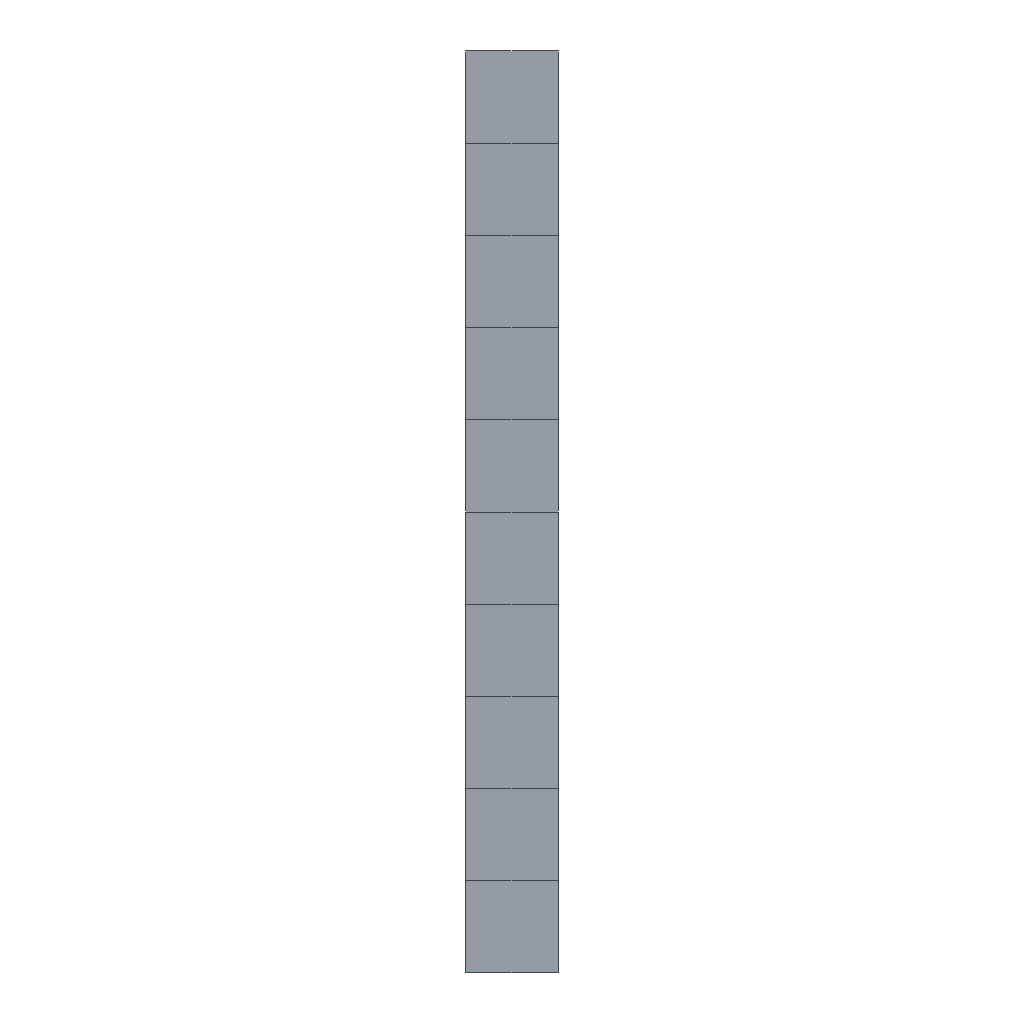Simulation study | abaqus
Set-up summary:
category,name,step,type,value,unit,region
solver,abaqus,,Abaqus/CAE 2024
units,mm-N-s-tonne (MPa),,inferred,E=10000 density=
analysis,load,,soils,time_period=0.001
analysis,consolidation,,soils,time_period=1.728e+06
mesh,nodes,,,22
mesh,elements,,,10
element_type,CPE4P,,,10
material,soil,,E,10000
material,soil,,nu,0.3
section,soil,,solid section,,,_PickedSet2
load,void,initial,initial condition ratio
load,Load-1,load,pressure,200,,_PickedSurf7
bc,BC-1,initial,fixed,[dofs=y],,_PickedSet4
bc,BC-2,initial,fixed,[dofs=x],,_PickedSet5
bc,BC-3,consolidation,fixed,[dofs=8],,_PickedSet6_PP_
Abaqus input file, long lists of numbers shortened:
*Heading
** Job name: deck Model name: Model-1
** Generated by: Abaqus/CAE 2024
*Preprint, echo=NO, model=NO, history=NO, contact=NO
**
** PARTS
**
*Part, name=soil
*Node
      1,           0.,           0.
      2,           1.,           0.
** (20 more lines like these left out)
*Element, type=CPE4P
 1,  1,  2,  4,  3
 2,  3,  4,  6,  5
** (8 more lines like these left out)
*Nset, nset=_PickedSet2, internal, generate
  1,  22,   1
*Elset, elset=_PickedSet2, internal, generate
  1,  10,   1
*Nset, nset=soil, generate
  1,  22,   1
*Elset, elset=soil, generate
  1,  10,   1
** Section: soil
*Solid Section, elset=_PickedSet2, material=soil
1.,
*End Part
**
**
** ASSEMBLY
**
*Assembly, name=Assembly
**
*Instance, name=soil-1, part=soil
*End Instance
**
*Nset, nset=_PickedSet4, internal, instance=soil-1
 1, 2
*Elset, elset=_PickedSet4, internal, instance=soil-1
 1,
*Nset, nset=_PickedSet5, internal, instance=soil-1, generate
  1,  22,   1
*Elset, elset=_PickedSet5, internal, instance=soil-1, generate
  1,  10,   1
*Nset, nset=_PickedSet6, internal, instance=soil-1
 21, 22
*Elset, elset=_PickedSet6, internal, instance=soil-1
 10,
*Elset, elset=__PickedSurf7_S3, internal, instance=soil-1
 10,
*Surface, type=ELEMENT, name=_PickedSurf7, internal
__PickedSurf7_S3, S3
*Nset, nset=_PickedSet6_PP_, internal, instance=soil-1
 21, 22
*End Assembly
**
** MATERIALS
**
*Material, name=soil
*Elastic
10000., 0.3
*Permeability, specific=10.
 1e-07, 1.5
**
** BOUNDARY CONDITIONS
**
** Name: BC-1 Type: Displacement/Rotation
*Boundary
_PickedSet4, 2, 2
** Name: BC-2 Type: Displacement/Rotation
*Boundary
_PickedSet5, 1, 1
**
** PREDEFINED FIELDS
**
** Name: void   Type: Void ratio
*Initial Conditions, TYPE=RATIO
soil-1.soil, 1.5
** ----------------------------------------------------------------
**
** STEP: load
**
*Step, name=load, nlgeom=NO
*Soils, consolidation, end=PERIOD, creep=none
0.001, 0.001, , ,
**
** LOADS
**
** Name: Load-1   Type: Pressure
*Dsload
_PickedSurf7, P, 200.
**
** OUTPUT REQUESTS
**
*Restart, write, frequency=0
*Print, solve=NO
**
** FIELD OUTPUT: F-Output-1
**
*Output, field, variable=PRESELECT
**
** HISTORY OUTPUT: H-Output-1
**
*Output, history, variable=PRESELECT
*End Step
** ----------------------------------------------------------------
**
** STEP: consolidation
**
*Step, name=consolidation, nlgeom=NO, inc=1000
*Soils, consolidation, end=SS, utol=200., creep=none
2000., 1.728e+06, 2000., 20000., 1e-05
**
** BOUNDARY CONDITIONS
**
** Name: BC-3 Type: Pore pressure
*Boundary
_PickedSet6_PP_, 8, 8
**
** OUTPUT REQUESTS
**
*Restart, write, frequency=0
**
** FIELD OUTPUT: F-Output-1
**
*Output, field, variable=PRESELECT
**
** HISTORY OUTPUT: H-Output-1
**
*Output, history, variable=PRESELECT
*End Step
Results summary:
result,odb.job_status,,,JOB_STATUS_COMPLETED_SUCCESSFULLY,"consistent, unstated (Abaqus has no unit system)"
result,steps[0].procedure,load,,"*SOILS, CONSOLIDATION","consistent, unstated (Abaqus has no unit system)"
result,steps[0].time_period,load,,0.001,"consistent, unstated (Abaqus has no unit system)"
result,steps[0].n_frames,load,,2,"consistent, unstated (Abaqus has no unit system)"
result,steps[0].last_frame.id,load,,1,"consistent, unstated (Abaqus has no unit system)"
result,steps[0].last_frame.value,load,,0.001,"consistent, unstated (Abaqus has no unit system)"
result,steps[0].last_frame.description,load,,Increment      1: Step Time =   1.0000E-03,"consistent, unstated (Abaqus has no unit system)"
result,steps[0].completed,load,,True,"consistent, unstated (Abaqus has no unit system)"
result,steps[0].max_U_magnitude,load,,2.31606e-18,"consistent, unstated (Abaqus has no unit system)"
result,steps[0].max_S_mises,load,,1.83801e-14,"consistent, unstated (Abaqus has no unit system)"
result,steps[0].RF_sum[1],load,,0,"consistent, unstated (Abaqus has no unit system)"
result,steps[0].RF_sum[2],load,,200,"consistent, unstated (Abaqus has no unit system)"
result,steps[1].procedure,consolidation,,"*SOILS, CONSOLIDATION","consistent, unstated (Abaqus has no unit system)"
result,steps[1].time_period,consolidation,,1.394e+06,"consistent, unstated (Abaqus has no unit system)"
result,steps[1].n_frames,consolidation,,75,"consistent, unstated (Abaqus has no unit system)"
result,steps[1].last_frame.id,consolidation,,74,"consistent, unstated (Abaqus has no unit system)"
result,steps[1].last_frame.value,consolidation,,1.394e+06,"consistent, unstated (Abaqus has no unit system)"
result,steps[1].last_frame.description,consolidation,,Increment     74: Step Time =   1.3940E+06,"consistent, unstated (Abaqus has no unit system)"
result,steps[1].completed,consolidation,,True,"consistent, unstated (Abaqus has no unit system)"
result,steps[1].max_U_magnitude,consolidation,,0.1472,"consistent, unstated (Abaqus has no unit system)"
result,steps[1].max_S_mises,consolidation,,114.159,"consistent, unstated (Abaqus has no unit system)"
result,steps[1].RF_sum[1],consolidation,,0,"consistent, unstated (Abaqus has no unit system)"
result,steps[1].RF_sum[2],consolidation,,200,"consistent, unstated (Abaqus has no unit system)"